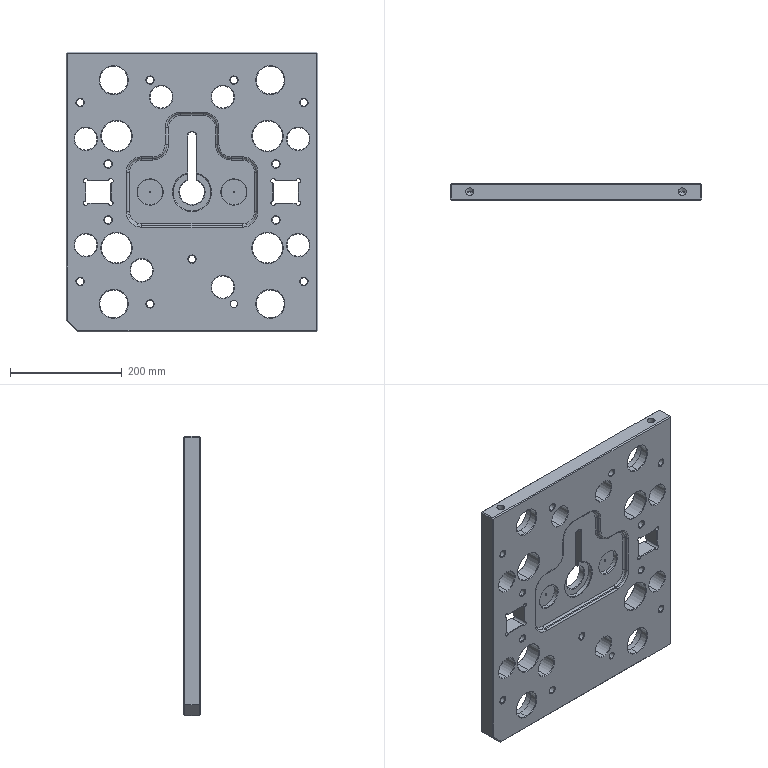Part | STEP file | Placa fechamento - MANIFOLD - Torre - 1 cav | 1 solid | 385 faces | box 450 x 30 x 500 mm | volume 5239142 mm3 | cylinder 148 | cone 134 | plane 87 | torus 16 | commonest cylinder face diameters 13 x26 20 x26 6 x16 40 x16 50 x16 8 x12